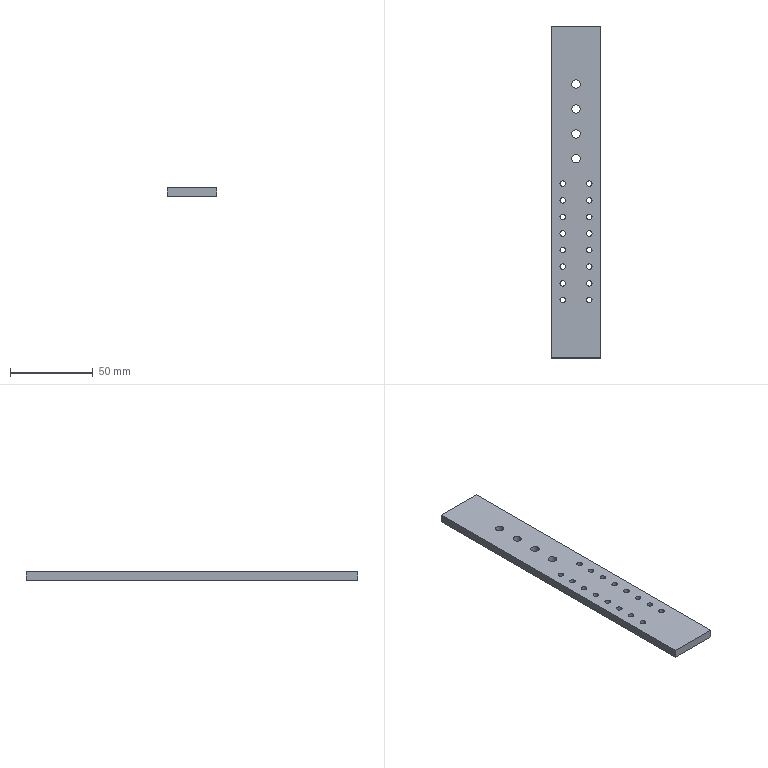Part | STEP file | Ground copper plate | 1 solid | 46 faces | box 30 x 200 x 5 mm | volume 28923 mm3 | cylinder 40 | plane 6 | commonest cylinder face diameters 3.3 x32 5 x8